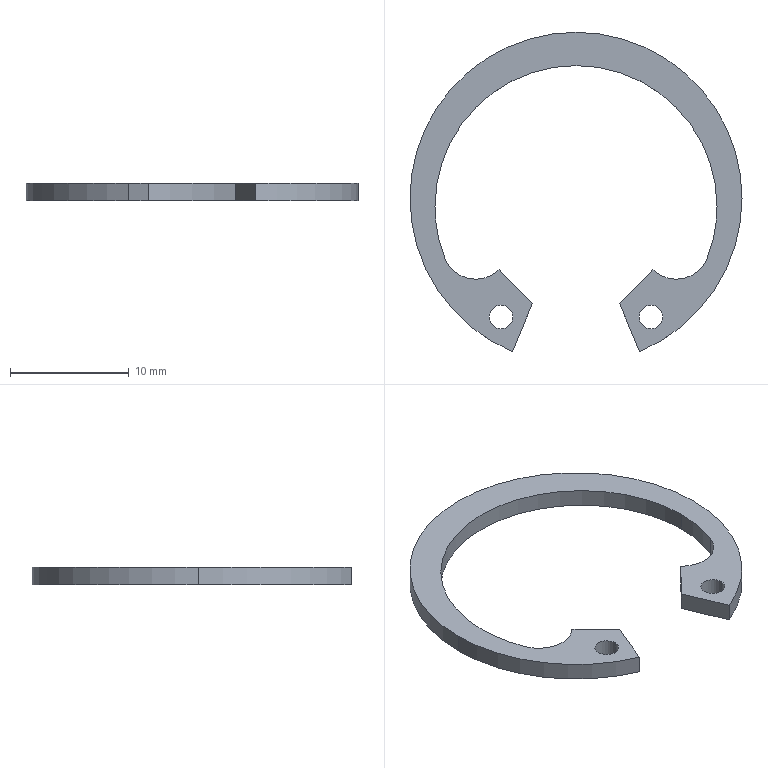Part | SolidWorks | features Extrusion 1 | 1 solid | 18 faces | box 27.9 x 26.838 x 1.5 mm | volume 279.179 mm3 | cylinder 12 | plane 6 | commonest cylinder face diameters 2 x4 23.7 x3 27.9 x3 5.6 x2
STEP:
#1=CARTESIAN_POINT('',(5.298,-9.979,1.5));
#2=VERTEX_POINT('',#1);
#3=CARTESIAN_POINT('',(7.298,-9.979,1.5));
#4=VERTEX_POINT('',#3);
#5=CARTESIAN_POINT('',(6.298,-9.979,1.5));
#6=DIRECTION('',(0.,0.,1.));
#7=DIRECTION('',(-1.,0.,0.));
#8=AXIS2_PLACEMENT_3D('',#5,#6,#7);
#9=CIRCLE('',#8,1.);
#10=EDGE_CURVE('',#2,#4,#9,.T.);
#11=ORIENTED_EDGE('',*,*,#10,.T.);
#12=CARTESIAN_POINT('',(7.298,-9.979,0.));
#13=VERTEX_POINT('',#12);
#14=CARTESIAN_POINT('',(7.298,-9.979,1.5));
#15=DIRECTION('',(0.,0.,-1.));
#16=VECTOR('',#15,1000.);
#17=LINE('',#14,#16);
#18=EDGE_CURVE('',#4,#13,#17,.T.);
#19=ORIENTED_EDGE('',*,*,#18,.T.);
#20=CARTESIAN_POINT('',(5.298,-9.979,0.));
#21=VERTEX_POINT('',#20);
#22=CARTESIAN_POINT('',(6.298,-9.979,0.));
#23=DIRECTION('',(0.,0.,1.));
#24=DIRECTION('',(-1.,0.,0.));
#25=AXIS2_PLACEMENT_3D('',#22,#23,#24);
#26=CIRCLE('',#25,1.);
#27=EDGE_CURVE('',#21,#13,#26,.T.);
#28=ORIENTED_EDGE('',*,*,#27,.F.);
#29=CARTESIAN_POINT('',(5.298,-9.979,1.5));
#30=DIRECTION('',(0.,0.,-1.));
#31=VECTOR('',#30,1000.);
#32=LINE('',#29,#31);
#33=EDGE_CURVE('',#2,#21,#32,.T.);
#34=ORIENTED_EDGE('',*,*,#33,.F.);
#35=EDGE_LOOP('',(#11,#19,#28,#34));
#36=FACE_OUTER_BOUND('',#35,.T.);
#37=CARTESIAN_POINT('',(6.298,-9.979,1.5));
#38=DIRECTION('',(0.,0.,-1.));
#39=DIRECTION('',(-1.,0.,0.));
#40=AXIS2_PLACEMENT_3D('',#37,#38,#39);
#41=CYLINDRICAL_SURFACE('',#40,1.);
#42=ADVANCED_FACE('',(#36),#41,.F.);
#43=CARTESIAN_POINT('',(-7.298,-9.979,1.5));
#44=VERTEX_POINT('',#43);
#45=CARTESIAN_POINT('',(-5.298,-9.979,1.5));
#46=VERTEX_POINT('',#45);
#47=CARTESIAN_POINT('',(-6.298,-9.979,1.5));
#48=DIRECTION('',(0.,0.,1.));
#49=DIRECTION('',(1.,0.,0.));
#50=AXIS2_PLACEMENT_3D('',#47,#48,#49);
#51=CIRCLE('',#50,1.);
#52=EDGE_CURVE('',#44,#46,#51,.T.);
#53=ORIENTED_EDGE('',*,*,#52,.T.);
#54=CARTESIAN_POINT('',(-5.298,-9.979,0.));
#55=VERTEX_POINT('',#54);
#56=CARTESIAN_POINT('',(-5.298,-9.979,1.5));
#57=DIRECTION('',(0.,0.,-1.));
#58=VECTOR('',#57,1000.);
#59=LINE('',#56,#58);
#60=EDGE_CURVE('',#46,#55,#59,.T.);
#61=ORIENTED_EDGE('',*,*,#60,.T.);
#62=CARTESIAN_POINT('',(-7.298,-9.979,0.));
#63=VERTEX_POINT('',#62);
#64=CARTESIAN_POINT('',(-6.298,-9.979,0.));
#65=DIRECTION('',(0.,0.,1.));
#66=DIRECTION('',(1.,0.,0.));
#67=AXIS2_PLACEMENT_3D('',#64,#65,#66);
#68=CIRCLE('',#67,1.);
#69=EDGE_CURVE('',#63,#55,#68,.T.);
#70=ORIENTED_EDGE('',*,*,#69,.F.);
#71=CARTESIAN_POINT('',(-7.298,-9.979,1.5));
#72=DIRECTION('',(0.,0.,-1.));
#73=VECTOR('',#72,1000.);
#74=LINE('',#71,#73);
#75=EDGE_CURVE('',#44,#63,#74,.T.);
#76=ORIENTED_EDGE('',*,*,#75,.F.);
#77=EDGE_LOOP('',(#53,#61,#70,#76));
#78=FACE_OUTER_BOUND('',#77,.T.);
#79=CARTESIAN_POINT('',(-6.298,-9.979,1.5));
#80=DIRECTION('',(0.,0.,-1.));
#81=DIRECTION('',(-1.,0.,0.));
#82=AXIS2_PLACEMENT_3D('',#79,#80,#81);
#83=CYLINDRICAL_SURFACE('',#82,1.);
#84=ADVANCED_FACE('',(#78),#83,.F.);
#85=CARTESIAN_POINT('',(11.85,-0.7,1.5));
#86=VERTEX_POINT('',#85);
#87=CARTESIAN_POINT('',(11.034,-5.022,1.5));
#88=VERTEX_POINT('',#87);
#89=CARTESIAN_POINT('',(0.,-0.7,1.5));
#90=DIRECTION('',(0.,0.,-1.));
#91=DIRECTION('',(1.,0.,0.));
#92=AXIS2_PLACEMENT_3D('',#89,#90,#91);
#93=CIRCLE('',#92,11.85);
#94=EDGE_CURVE('',#86,#88,#93,.T.);
#95=ORIENTED_EDGE('',*,*,#94,.F.);
#96=CARTESIAN_POINT('',(11.85,-0.7,0.));
#97=VERTEX_POINT('',#96);
#98=CARTESIAN_POINT('',(11.85,-0.7,1.5));
#99=DIRECTION('',(0.,0.,-1.));
#100=VECTOR('',#99,1000.);
#101=LINE('',#98,#100);
#102=EDGE_CURVE('',#86,#97,#101,.T.);
#103=ORIENTED_EDGE('',*,*,#102,.T.);
#104=CARTESIAN_POINT('',(11.034,-5.022,0.));
#105=VERTEX_POINT('',#104);
#106=CARTESIAN_POINT('',(0.,-0.7,0.));
#107=DIRECTION('',(0.,0.,-1.));
#108=DIRECTION('',(1.,0.,0.));
#109=AXIS2_PLACEMENT_3D('',#106,#107,#108);
#110=CIRCLE('',#109,11.85);
#111=EDGE_CURVE('',#97,#105,#110,.T.);
#112=ORIENTED_EDGE('',*,*,#111,.T.);
#113=CARTESIAN_POINT('',(11.034,-5.022,1.5));
#114=DIRECTION('',(0.,0.,-1.));
#115=VECTOR('',#114,1000.);
#116=LINE('',#113,#115);
#117=EDGE_CURVE('',#88,#105,#116,.T.);
#118=ORIENTED_EDGE('',*,*,#117,.F.);
#119=EDGE_LOOP('',(#95,#103,#112,#118));
#120=FACE_OUTER_BOUND('',#119,.T.);
#121=CARTESIAN_POINT('',(0.,-0.7,1.5));
#122=DIRECTION('',(0.,0.,-1.));
#123=DIRECTION('',(-1.,0.,0.));
#124=AXIS2_PLACEMENT_3D('',#121,#122,#123);
#125=CYLINDRICAL_SURFACE('',#124,11.85);
#126=ADVANCED_FACE('',(#120),#125,.F.);
#127=ORIENTED_EDGE('',*,*,#102,.F.);
#128=CARTESIAN_POINT('',(-11.85,-0.7,1.5));
#129=VERTEX_POINT('',#128);
#130=CARTESIAN_POINT('',(0.,-0.7,1.5));
#131=DIRECTION('',(0.,0.,-1.));
#132=DIRECTION('',(1.,0.,0.));
#133=AXIS2_PLACEMENT_3D('',#130,#131,#132);
#134=CIRCLE('',#133,11.85);
#135=EDGE_CURVE('',#129,#86,#134,.T.);
#136=ORIENTED_EDGE('',*,*,#135,.F.);
#137=CARTESIAN_POINT('',(-11.85,-0.7,0.));
#138=VERTEX_POINT('',#137);
#139=CARTESIAN_POINT('',(-11.85,-0.7,1.5));
#140=DIRECTION('',(0.,0.,-1.));
#141=VECTOR('',#140,1000.);
#142=LINE('',#139,#141);
#143=EDGE_CURVE('',#129,#138,#142,.T.);
#144=ORIENTED_EDGE('',*,*,#143,.T.);
#145=CARTESIAN_POINT('',(0.,-0.7,0.));
#146=DIRECTION('',(0.,0.,-1.));
#147=DIRECTION('',(1.,0.,0.));
#148=AXIS2_PLACEMENT_3D('',#145,#146,#147);
#149=CIRCLE('',#148,11.85);
#150=EDGE_CURVE('',#138,#97,#149,.T.);
#151=ORIENTED_EDGE('',*,*,#150,.T.);
#152=EDGE_LOOP('',(#127,#136,#144,#151));
#153=FACE_OUTER_BOUND('',#152,.T.);
#154=CARTESIAN_POINT('',(0.,-0.7,1.5));
#155=DIRECTION('',(0.,0.,-1.));
#156=DIRECTION('',(-1.,0.,0.));
#157=AXIS2_PLACEMENT_3D('',#154,#155,#156);
#158=CYLINDRICAL_SURFACE('',#157,11.85);
#159=ADVANCED_FACE('',(#153),#158,.F.);
#160=CARTESIAN_POINT('',(13.95,0.,1.5));
#161=VERTEX_POINT('',#160);
#162=CARTESIAN_POINT('',(-13.95,0.,1.5));
#163=VERTEX_POINT('',#162);
#164=CARTESIAN_POINT('',(0.,0.,1.5));
#165=DIRECTION('',(0.,0.,1.));
#166=DIRECTION('',(1.,0.,0.));
#167=AXIS2_PLACEMENT_3D('',#164,#165,#166);
#168=CIRCLE('',#167,13.95);
#169=EDGE_CURVE('',#161,#163,#168,.T.);
#170=ORIENTED_EDGE('',*,*,#169,.F.);
#171=CARTESIAN_POINT('',(13.95,0.,0.));
#172=VERTEX_POINT('',#171);
#173=CARTESIAN_POINT('',(13.95,0.,1.5));
#174=DIRECTION('',(0.,0.,-1.));
#175=VECTOR('',#174,1000.);
#176=LINE('',#173,#175);
#177=EDGE_CURVE('',#161,#172,#176,.T.);
#178=ORIENTED_EDGE('',*,*,#177,.T.);
#179=CARTESIAN_POINT('',(-13.95,0.,0.));
#180=VERTEX_POINT('',#179);
#181=CARTESIAN_POINT('',(0.,0.,0.));
#182=DIRECTION('',(0.,0.,1.));
#183=DIRECTION('',(1.,0.,0.));
#184=AXIS2_PLACEMENT_3D('',#181,#182,#183);
#185=CIRCLE('',#184,13.95);
#186=EDGE_CURVE('',#172,#180,#185,.T.);
#187=ORIENTED_EDGE('',*,*,#186,.T.);
#188=CARTESIAN_POINT('',(-13.95,0.,1.5));
#189=DIRECTION('',(0.,0.,-1.));
#190=VECTOR('',#189,1000.);
#191=LINE('',#188,#190);
#192=EDGE_CURVE('',#163,#180,#191,.T.);
#193=ORIENTED_EDGE('',*,*,#192,.F.);
#194=EDGE_LOOP('',(#170,#178,#187,#193));
#195=FACE_OUTER_BOUND('',#194,.T.);
#196=CARTESIAN_POINT('',(0.,0.,1.5));
#197=DIRECTION('',(0.,0.,-1.));
#198=DIRECTION('',(-1.,0.,0.));
#199=AXIS2_PLACEMENT_3D('',#196,#197,#198);
#200=CYLINDRICAL_SURFACE('',#199,13.95);
#201=ADVANCED_FACE('',(#195),#200,.T.);
#202=CARTESIAN_POINT('',(-5.338,-12.888,1.5));
#203=VERTEX_POINT('',#202);
#204=CARTESIAN_POINT('',(0.,0.,1.5));
#205=DIRECTION('',(0.,0.,1.));
#206=DIRECTION('',(1.,0.,0.));
#207=AXIS2_PLACEMENT_3D('',#204,#205,#206);
#208=CIRCLE('',#207,13.95);
#209=EDGE_CURVE('',#163,#203,#208,.T.);
#210=ORIENTED_EDGE('',*,*,#209,.F.);
#211=ORIENTED_EDGE('',*,*,#192,.T.);
#212=CARTESIAN_POINT('',(-5.338,-12.888,0.));
#213=VERTEX_POINT('',#212);
#214=CARTESIAN_POINT('',(0.,0.,0.));
#215=DIRECTION('',(0.,0.,1.));
#216=DIRECTION('',(1.,0.,0.));
#217=AXIS2_PLACEMENT_3D('',#214,#215,#216);
#218=CIRCLE('',#217,13.95);
#219=EDGE_CURVE('',#180,#213,#218,.T.);
#220=ORIENTED_EDGE('',*,*,#219,.T.);
#221=CARTESIAN_POINT('',(-5.338,-12.888,1.5));
#222=DIRECTION('',(0.,0.,-1.));
#223=VECTOR('',#222,1000.);
#224=LINE('',#221,#223);
#225=EDGE_CURVE('',#203,#213,#224,.T.);
#226=ORIENTED_EDGE('',*,*,#225,.F.);
#227=EDGE_LOOP('',(#210,#211,#220,#226));
#228=FACE_OUTER_BOUND('',#227,.T.);
#229=CARTESIAN_POINT('',(0.,0.,1.5));
#230=DIRECTION('',(0.,0.,-1.));
#231=DIRECTION('',(-1.,0.,0.));
#232=AXIS2_PLACEMENT_3D('',#229,#230,#231);
#233=CYLINDRICAL_SURFACE('',#232,13.95);
#234=ADVANCED_FACE('',(#228),#233,.T.);
#235=ORIENTED_EDGE('',*,*,#52,.F.);
#236=CARTESIAN_POINT('',(-6.298,-9.979,1.5));
#237=DIRECTION('',(0.,0.,1.));
#238=DIRECTION('',(1.,0.,0.));
#239=AXIS2_PLACEMENT_3D('',#236,#237,#238);
#240=CIRCLE('',#239,1.);
#241=EDGE_CURVE('',#46,#44,#240,.T.);
#242=ORIENTED_EDGE('',*,*,#241,.F.);
#243=EDGE_LOOP('',(#235,#242));
#244=FACE_BOUND('',#243,.T.);
#245=CARTESIAN_POINT('',(5.338,-12.888,1.5));
#246=VERTEX_POINT('',#245);
#247=CARTESIAN_POINT('',(0.,0.,1.5));
#248=DIRECTION('',(0.,0.,1.));
#249=DIRECTION('',(1.,0.,0.));
#250=AXIS2_PLACEMENT_3D('',#247,#248,#249);
#251=CIRCLE('',#250,13.95);
#252=EDGE_CURVE('',#246,#161,#251,.T.);
#253=ORIENTED_EDGE('',*,*,#252,.T.);
#254=ORIENTED_EDGE('',*,*,#169,.T.);
#255=ORIENTED_EDGE('',*,*,#209,.T.);
#256=CARTESIAN_POINT('',(-3.67,-8.86,1.5));
#257=VERTEX_POINT('',#256);
#258=CARTESIAN_POINT('',(-3.67,-8.86,1.5));
#259=DIRECTION('',(0.3827,0.9239,0.));
#260=VECTOR('',#259,1000.);
#261=LINE('',#258,#260);
#262=EDGE_CURVE('',#203,#257,#261,.T.);
#263=ORIENTED_EDGE('',*,*,#262,.T.);
#264=CARTESIAN_POINT('',(-6.468,-6.002,1.5));
#265=VERTEX_POINT('',#264);
#266=CARTESIAN_POINT('',(-6.468,-6.002,1.5));
#267=DIRECTION('',(-0.6995,0.7146,0.));
#268=VECTOR('',#267,1000.);
#269=LINE('',#266,#268);
#270=EDGE_CURVE('',#257,#265,#269,.T.);
#271=ORIENTED_EDGE('',*,*,#270,.T.);
#272=CARTESIAN_POINT('',(-11.034,-5.022,1.5));
#273=VERTEX_POINT('',#272);
#274=CARTESIAN_POINT('',(-8.427,-4.001,1.5));
#275=DIRECTION('',(0.,0.,-1.));
#276=DIRECTION('',(1.,0.,0.));
#277=AXIS2_PLACEMENT_3D('',#274,#275,#276);
#278=CIRCLE('',#277,2.8);
#279=EDGE_CURVE('',#265,#273,#278,.T.);
#280=ORIENTED_EDGE('',*,*,#279,.T.);
#281=CARTESIAN_POINT('',(0.,-0.7,1.5));
#282=DIRECTION('',(0.,0.,-1.));
#283=DIRECTION('',(1.,0.,0.));
#284=AXIS2_PLACEMENT_3D('',#281,#282,#283);
#285=CIRCLE('',#284,11.85);
#286=EDGE_CURVE('',#273,#129,#285,.T.);
#287=ORIENTED_EDGE('',*,*,#286,.T.);
#288=ORIENTED_EDGE('',*,*,#135,.T.);
#289=ORIENTED_EDGE('',*,*,#94,.T.);
#290=CARTESIAN_POINT('',(6.468,-6.002,1.5));
#291=VERTEX_POINT('',#290);
#292=CARTESIAN_POINT('',(8.427,-4.001,1.5));
#293=DIRECTION('',(0.,0.,-1.));
#294=DIRECTION('',(-1.,0.,0.));
#295=AXIS2_PLACEMENT_3D('',#292,#293,#294);
#296=CIRCLE('',#295,2.8);
#297=EDGE_CURVE('',#88,#291,#296,.T.);
#298=ORIENTED_EDGE('',*,*,#297,.T.);
#299=CARTESIAN_POINT('',(3.67,-8.86,1.5));
#300=VERTEX_POINT('',#299);
#301=CARTESIAN_POINT('',(6.468,-6.002,1.5));
#302=DIRECTION('',(-0.6995,-0.7146,0.));
#303=VECTOR('',#302,1000.);
#304=LINE('',#301,#303);
#305=EDGE_CURVE('',#291,#300,#304,.T.);
#306=ORIENTED_EDGE('',*,*,#305,.T.);
#307=CARTESIAN_POINT('',(3.67,-8.86,1.5));
#308=DIRECTION('',(0.3827,-0.9239,0.));
#309=VECTOR('',#308,1000.);
#310=LINE('',#307,#309);
#311=EDGE_CURVE('',#300,#246,#310,.T.);
#312=ORIENTED_EDGE('',*,*,#311,.T.);
#313=EDGE_LOOP('',(#253,#254,#255,#263,#271,#280,#287,#288,#289,#298,#306,#312));
#314=FACE_OUTER_BOUND('',#313,.T.);
#315=ORIENTED_EDGE('',*,*,#10,.F.);
#316=CARTESIAN_POINT('',(6.298,-9.979,1.5));
#317=DIRECTION('',(0.,0.,1.));
#318=DIRECTION('',(-1.,0.,0.));
#319=AXIS2_PLACEMENT_3D('',#316,#317,#318);
#320=CIRCLE('',#319,1.);
#321=EDGE_CURVE('',#4,#2,#320,.T.);
#322=ORIENTED_EDGE('',*,*,#321,.F.);
#323=EDGE_LOOP('',(#315,#322));
#324=FACE_BOUND('',#323,.T.);
#325=CARTESIAN_POINT('',(0.,0.,1.5));
#326=DIRECTION('',(0.,0.,1.));
#327=DIRECTION('',(1.,0.,0.));
#328=AXIS2_PLACEMENT_3D('',#325,#326,#327);
#329=PLANE('',#328);
#330=ADVANCED_FACE('',(#244,#314,#324),#329,.T.);
#331=CARTESIAN_POINT('',(5.338,-12.888,0.));
#332=VERTEX_POINT('',#331);
#333=CARTESIAN_POINT('',(0.,0.,0.));
#334=DIRECTION('',(0.,0.,1.));
#335=DIRECTION('',(1.,0.,0.));
#336=AXIS2_PLACEMENT_3D('',#333,#334,#335);
#337=CIRCLE('',#336,13.95);
#338=EDGE_CURVE('',#332,#172,#337,.T.);
#339=ORIENTED_EDGE('',*,*,#338,.F.);
#340=CARTESIAN_POINT('',(3.67,-8.86,0.));
#341=VERTEX_POINT('',#340);
#342=CARTESIAN_POINT('',(3.67,-8.86,0.));
#343=DIRECTION('',(0.3827,-0.9239,0.));
#344=VECTOR('',#343,1000.);
#345=LINE('',#342,#344);
#346=EDGE_CURVE('',#341,#332,#345,.T.);
#347=ORIENTED_EDGE('',*,*,#346,.F.);
#348=CARTESIAN_POINT('',(6.468,-6.002,0.));
#349=VERTEX_POINT('',#348);
#350=CARTESIAN_POINT('',(6.468,-6.002,0.));
#351=DIRECTION('',(-0.6995,-0.7146,0.));
#352=VECTOR('',#351,1000.);
#353=LINE('',#350,#352);
#354=EDGE_CURVE('',#349,#341,#353,.T.);
#355=ORIENTED_EDGE('',*,*,#354,.F.);
#356=CARTESIAN_POINT('',(8.427,-4.001,0.));
#357=DIRECTION('',(0.,0.,-1.));
#358=DIRECTION('',(-1.,0.,0.));
#359=AXIS2_PLACEMENT_3D('',#356,#357,#358);
#360=CIRCLE('',#359,2.8);
#361=EDGE_CURVE('',#105,#349,#360,.T.);
#362=ORIENTED_EDGE('',*,*,#361,.F.);
#363=ORIENTED_EDGE('',*,*,#111,.F.);
#364=ORIENTED_EDGE('',*,*,#150,.F.);
#365=CARTESIAN_POINT('',(-11.034,-5.022,0.));
#366=VERTEX_POINT('',#365);
#367=CARTESIAN_POINT('',(0.,-0.7,0.));
#368=DIRECTION('',(0.,0.,-1.));
#369=DIRECTION('',(1.,0.,0.));
#370=AXIS2_PLACEMENT_3D('',#367,#368,#369);
#371=CIRCLE('',#370,11.85);
#372=EDGE_CURVE('',#366,#138,#371,.T.);
#373=ORIENTED_EDGE('',*,*,#372,.F.);
#374=CARTESIAN_POINT('',(-6.468,-6.002,0.));
#375=VERTEX_POINT('',#374);
#376=CARTESIAN_POINT('',(-8.427,-4.001,0.));
#377=DIRECTION('',(0.,0.,-1.));
#378=DIRECTION('',(1.,0.,0.));
#379=AXIS2_PLACEMENT_3D('',#376,#377,#378);
#380=CIRCLE('',#379,2.8);
#381=EDGE_CURVE('',#375,#366,#380,.T.);
#382=ORIENTED_EDGE('',*,*,#381,.F.);
#383=CARTESIAN_POINT('',(-3.67,-8.86,0.));
#384=VERTEX_POINT('',#383);
#385=CARTESIAN_POINT('',(-6.468,-6.002,0.));
#386=DIRECTION('',(-0.6995,0.7146,0.));
#387=VECTOR('',#386,1000.);
#388=LINE('',#385,#387);
#389=EDGE_CURVE('',#384,#375,#388,.T.);
#390=ORIENTED_EDGE('',*,*,#389,.F.);
#391=CARTESIAN_POINT('',(-3.67,-8.86,0.));
#392=DIRECTION('',(0.3827,0.9239,0.));
#393=VECTOR('',#392,1000.);
#394=LINE('',#391,#393);
#395=EDGE_CURVE('',#213,#384,#394,.T.);
#396=ORIENTED_EDGE('',*,*,#395,.F.);
#397=ORIENTED_EDGE('',*,*,#219,.F.);
#398=ORIENTED_EDGE('',*,*,#186,.F.);
#399=EDGE_LOOP('',(#339,#347,#355,#362,#363,#364,#373,#382,#390,#396,#397,#398));
#400=FACE_OUTER_BOUND('',#399,.T.);
#401=ORIENTED_EDGE('',*,*,#69,.T.);
#402=CARTESIAN_POINT('',(-6.298,-9.979,0.));
#403=DIRECTION('',(0.,0.,1.));
#404=DIRECTION('',(1.,0.,0.));
#405=AXIS2_PLACEMENT_3D('',#402,#403,#404);
#406=CIRCLE('',#405,1.);
#407=EDGE_CURVE('',#55,#63,#406,.T.);
#408=ORIENTED_EDGE('',*,*,#407,.T.);
#409=EDGE_LOOP('',(#401,#408));
#410=FACE_BOUND('',#409,.T.);
#411=ORIENTED_EDGE('',*,*,#27,.T.);
#412=CARTESIAN_POINT('',(6.298,-9.979,0.));
#413=DIRECTION('',(0.,0.,1.));
#414=DIRECTION('',(-1.,0.,0.));
#415=AXIS2_PLACEMENT_3D('',#412,#413,#414);
#416=CIRCLE('',#415,1.);
#417=EDGE_CURVE('',#13,#21,#416,.T.);
#418=ORIENTED_EDGE('',*,*,#417,.T.);
#419=EDGE_LOOP('',(#411,#418));
#420=FACE_BOUND('',#419,.T.);
#421=CARTESIAN_POINT('',(0.,0.,0.));
#422=DIRECTION('',(0.,0.,1.));
#423=DIRECTION('',(1.,0.,0.));
#424=AXIS2_PLACEMENT_3D('',#421,#422,#423);
#425=PLANE('',#424);
#426=ADVANCED_FACE('',(#400,#410,#420),#425,.F.);
#427=ORIENTED_EDGE('',*,*,#177,.F.);
#428=ORIENTED_EDGE('',*,*,#252,.F.);
#429=CARTESIAN_POINT('',(5.338,-12.888,1.5));
#430=DIRECTION('',(0.,0.,-1.));
#431=VECTOR('',#430,1000.);
#432=LINE('',#429,#431);
#433=EDGE_CURVE('',#246,#332,#432,.T.);
#434=ORIENTED_EDGE('',*,*,#433,.T.);
#435=ORIENTED_EDGE('',*,*,#338,.T.);
#436=EDGE_LOOP('',(#427,#428,#434,#435));
#437=FACE_OUTER_BOUND('',#436,.T.);
#438=CARTESIAN_POINT('',(0.,0.,1.5));
#439=DIRECTION('',(0.,0.,-1.));
#440=DIRECTION('',(-1.,0.,0.));
#441=AXIS2_PLACEMENT_3D('',#438,#439,#440);
#442=CYLINDRICAL_SURFACE('',#441,13.95);
#443=ADVANCED_FACE('',(#437),#442,.T.);
#444=ORIENTED_EDGE('',*,*,#395,.T.);
#445=CARTESIAN_POINT('',(-3.67,-8.86,1.5));
#446=DIRECTION('',(0.,0.,-1.));
#447=VECTOR('',#446,1000.);
#448=LINE('',#445,#447);
#449=EDGE_CURVE('',#257,#384,#448,.T.);
#450=ORIENTED_EDGE('',*,*,#449,.F.);
#451=ORIENTED_EDGE('',*,*,#262,.F.);
#452=ORIENTED_EDGE('',*,*,#225,.T.);
#453=EDGE_LOOP('',(#444,#450,#451,#452));
#454=FACE_OUTER_BOUND('',#453,.T.);
#455=CARTESIAN_POINT('',(-3.67,-8.86,1.5));
#456=DIRECTION('',(-0.9239,0.3827,0.));
#457=DIRECTION('',(-0.3827,-0.9239,0.));
#458=AXIS2_PLACEMENT_3D('',#455,#456,#457);
#459=PLANE('',#458);
#460=ADVANCED_FACE('',(#454),#459,.F.);
#461=ORIENTED_EDGE('',*,*,#389,.T.);
#462=CARTESIAN_POINT('',(-6.468,-6.002,1.5));
#463=DIRECTION('',(0.,0.,-1.));
#464=VECTOR('',#463,1000.);
#465=LINE('',#462,#464);
#466=EDGE_CURVE('',#265,#375,#465,.T.);
#467=ORIENTED_EDGE('',*,*,#466,.F.);
#468=ORIENTED_EDGE('',*,*,#270,.F.);
#469=ORIENTED_EDGE('',*,*,#449,.T.);
#470=EDGE_LOOP('',(#461,#467,#468,#469));
#471=FACE_OUTER_BOUND('',#470,.T.);
#472=CARTESIAN_POINT('',(-6.468,-6.002,1.5));
#473=DIRECTION('',(-0.7146,-0.6995,0.));
#474=DIRECTION('',(0.6995,-0.7146,0.));
#475=AXIS2_PLACEMENT_3D('',#472,#473,#474);
#476=PLANE('',#475);
#477=ADVANCED_FACE('',(#471),#476,.F.);
#478=ORIENTED_EDGE('',*,*,#381,.T.);
#479=CARTESIAN_POINT('',(-11.034,-5.022,1.5));
#480=DIRECTION('',(0.,0.,-1.));
#481=VECTOR('',#480,1000.);
#482=LINE('',#479,#481);
#483=EDGE_CURVE('',#273,#366,#482,.T.);
#484=ORIENTED_EDGE('',*,*,#483,.F.);
#485=ORIENTED_EDGE('',*,*,#279,.F.);
#486=ORIENTED_EDGE('',*,*,#466,.T.);
#487=EDGE_LOOP('',(#478,#484,#485,#486));
#488=FACE_OUTER_BOUND('',#487,.T.);
#489=CARTESIAN_POINT('',(-8.427,-4.001,1.5));
#490=DIRECTION('',(0.,0.,-1.));
#491=DIRECTION('',(-1.,0.,0.));
#492=AXIS2_PLACEMENT_3D('',#489,#490,#491);
#493=CYLINDRICAL_SURFACE('',#492,2.8);
#494=ADVANCED_FACE('',(#488),#493,.F.);
#495=ORIENTED_EDGE('',*,*,#143,.F.);
#496=ORIENTED_EDGE('',*,*,#286,.F.);
#497=ORIENTED_EDGE('',*,*,#483,.T.);
#498=ORIENTED_EDGE('',*,*,#372,.T.);
#499=EDGE_LOOP('',(#495,#496,#497,#498));
#500=FACE_OUTER_BOUND('',#499,.T.);
#501=CARTESIAN_POINT('',(0.,-0.7,1.5));
#502=DIRECTION('',(0.,0.,-1.));
#503=DIRECTION('',(-1.,0.,0.));
#504=AXIS2_PLACEMENT_3D('',#501,#502,#503);
#505=CYLINDRICAL_SURFACE('',#504,11.85);
#506=ADVANCED_FACE('',(#500),#505,.F.);
#507=ORIENTED_EDGE('',*,*,#361,.T.);
#508=CARTESIAN_POINT('',(6.468,-6.002,1.5));
#509=DIRECTION('',(0.,0.,-1.));
#510=VECTOR('',#509,1000.);
#511=LINE('',#508,#510);
#512=EDGE_CURVE('',#291,#349,#511,.T.);
#513=ORIENTED_EDGE('',*,*,#512,.F.);
#514=ORIENTED_EDGE('',*,*,#297,.F.);
#515=ORIENTED_EDGE('',*,*,#117,.T.);
#516=EDGE_LOOP('',(#507,#513,#514,#515));
#517=FACE_OUTER_BOUND('',#516,.T.);
#518=CARTESIAN_POINT('',(8.427,-4.001,1.5));
#519=DIRECTION('',(0.,0.,-1.));
#520=DIRECTION('',(-1.,0.,0.));
#521=AXIS2_PLACEMENT_3D('',#518,#519,#520);
#522=CYLINDRICAL_SURFACE('',#521,2.8);
#523=ADVANCED_FACE('',(#517),#522,.F.);
#524=ORIENTED_EDGE('',*,*,#354,.T.);
#525=CARTESIAN_POINT('',(3.67,-8.86,1.5));
#526=DIRECTION('',(0.,0.,-1.));
#527=VECTOR('',#526,1000.);
#528=LINE('',#525,#527);
#529=EDGE_CURVE('',#300,#341,#528,.T.);
#530=ORIENTED_EDGE('',*,*,#529,.F.);
#531=ORIENTED_EDGE('',*,*,#305,.F.);
#532=ORIENTED_EDGE('',*,*,#512,.T.);
#533=EDGE_LOOP('',(#524,#530,#531,#532));
#534=FACE_OUTER_BOUND('',#533,.T.);
#535=CARTESIAN_POINT('',(6.468,-6.002,1.5));
#536=DIRECTION('',(0.7146,-0.6995,0.));
#537=DIRECTION('',(0.6995,0.7146,0.));
#538=AXIS2_PLACEMENT_3D('',#535,#536,#537);
#539=PLANE('',#538);
#540=ADVANCED_FACE('',(#534),#539,.F.);
#541=ORIENTED_EDGE('',*,*,#346,.T.);
#542=ORIENTED_EDGE('',*,*,#433,.F.);
#543=ORIENTED_EDGE('',*,*,#311,.F.);
#544=ORIENTED_EDGE('',*,*,#529,.T.);
#545=EDGE_LOOP('',(#541,#542,#543,#544));
#546=FACE_OUTER_BOUND('',#545,.T.);
#547=CARTESIAN_POINT('',(3.67,-8.86,1.5));
#548=DIRECTION('',(0.9239,0.3827,0.));
#549=DIRECTION('',(-0.3827,0.9239,0.));
#550=AXIS2_PLACEMENT_3D('',#547,#548,#549);
#551=PLANE('',#550);
#552=ADVANCED_FACE('',(#546),#551,.F.);
#553=ORIENTED_EDGE('',*,*,#60,.F.);
#554=ORIENTED_EDGE('',*,*,#241,.T.);
#555=ORIENTED_EDGE('',*,*,#75,.T.);
#556=ORIENTED_EDGE('',*,*,#407,.F.);
#557=EDGE_LOOP('',(#553,#554,#555,#556));
#558=FACE_OUTER_BOUND('',#557,.T.);
#559=CARTESIAN_POINT('',(-6.298,-9.979,1.5));
#560=DIRECTION('',(0.,0.,-1.));
#561=DIRECTION('',(-1.,0.,0.));
#562=AXIS2_PLACEMENT_3D('',#559,#560,#561);
#563=CYLINDRICAL_SURFACE('',#562,1.);
#564=ADVANCED_FACE('',(#558),#563,.F.);
#565=ORIENTED_EDGE('',*,*,#18,.F.);
#566=ORIENTED_EDGE('',*,*,#321,.T.);
#567=ORIENTED_EDGE('',*,*,#33,.T.);
#568=ORIENTED_EDGE('',*,*,#417,.F.);
#569=EDGE_LOOP('',(#565,#566,#567,#568));
#570=FACE_OUTER_BOUND('',#569,.T.);
#571=CARTESIAN_POINT('',(6.298,-9.979,1.5));
#572=DIRECTION('',(0.,0.,-1.));
#573=DIRECTION('',(-1.,0.,0.));
#574=AXIS2_PLACEMENT_3D('',#571,#572,#573);
#575=CYLINDRICAL_SURFACE('',#574,1.);
#576=ADVANCED_FACE('',(#570),#575,.F.);
#577=CLOSED_SHELL('',(#42,#84,#126,#159,#201,#234,#330,#426,#443,#460,#477,#494,#506,#523,#540,#552,#564,#576));
#578=MANIFOLD_SOLID_BREP('',#577);
#579=CARTESIAN_POINT('',(0.,0.,0.));
#580=DIRECTION('',(0.,0.,1.));
#581=DIRECTION('',(1.,0.,0.));
#582=AXIS2_PLACEMENT_3D('',#579,#580,#581);
#583=(LENGTH_UNIT()NAMED_UNIT(*)SI_UNIT(.MILLI.,.METRE.));
#584=UNCERTAINTY_MEASURE_WITH_UNIT(LENGTH_MEASURE(0.00001),#583,'','');
#585=(NAMED_UNIT(*)PLANE_ANGLE_UNIT()SI_UNIT($,.RADIAN.));
#586=(NAMED_UNIT(*)SI_UNIT($,.STERADIAN.)SOLID_ANGLE_UNIT());
#587=(GEOMETRIC_REPRESENTATION_CONTEXT(3)GLOBAL_UNCERTAINTY_ASSIGNED_CONTEXT((#584))GLOBAL_UNIT_ASSIGNED_CONTEXT((#583,#585,#586))REPRESENTATION_CONTEXT('',''));
#588=ADVANCED_BREP_SHAPE_REPRESENTATION('',(#578,#582),#587);